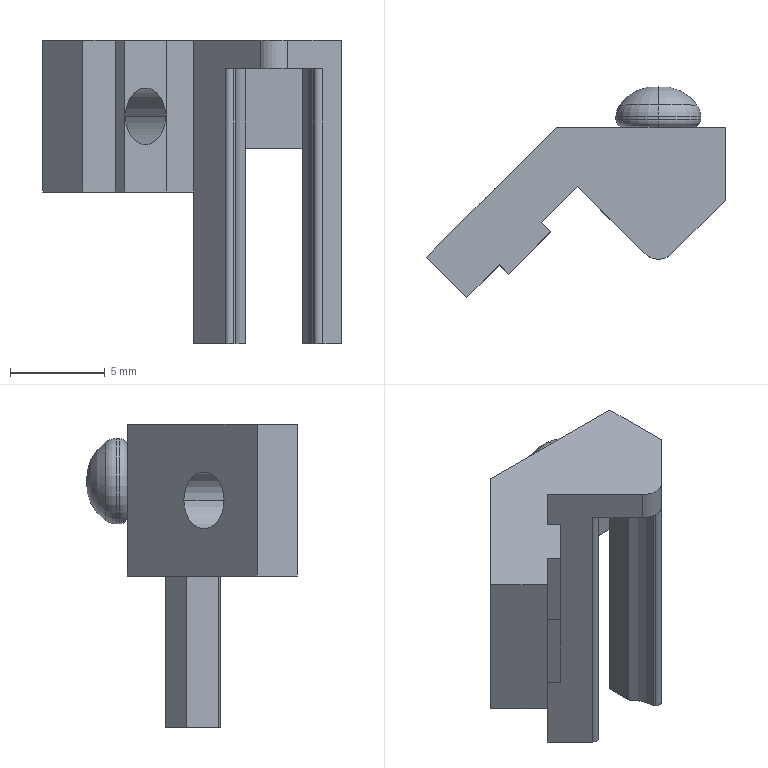Part | SolidWorks | features RefAxis 6, ICE 4, 3DProfileFeature 2, Extrusion 1, RevCut 1, Revolution 1 | 1 solid | 43 faces | box 15.769 x 11.133 x 16 mm | volume 523.118 mm3 | plane 28 | cylinder 9 | torus 6 | commonest cylinder face diameters 0.6 x2 3 x2 4.15 x2 4.5 x2 2 x1
STEP:
#1=CARTESIAN_POINT('',(0.,7.04,-1.5));
#2=VERTEX_POINT('',#1);
#3=CARTESIAN_POINT('',(0.,6.061,-3.557));
#4=VERTEX_POINT('',#3);
#5=CARTESIAN_POINT('',(0.,4.642,-1.62));
#6=DIRECTION('',(-1.,0.,0.));
#7=DIRECTION('',(0.,0.,1.));
#8=AXIS2_PLACEMENT_3D('',#5,#6,#7);
#9=CIRCLE('',#8,2.401);
#10=EDGE_CURVE('',#2,#4,#9,.T.);
#11=ORIENTED_EDGE('',*,*,#10,.F.);
#12=CARTESIAN_POINT('',(0.,6.061,0.5566));
#13=VERTEX_POINT('',#12);
#14=CARTESIAN_POINT('',(0.,4.642,-1.38));
#15=DIRECTION('',(1.,0.,0.));
#16=DIRECTION('',(0.,0.,-1.));
#17=AXIS2_PLACEMENT_3D('',#14,#15,#16);
#18=CIRCLE('',#17,2.401);
#19=EDGE_CURVE('',#2,#13,#18,.T.);
#20=ORIENTED_EDGE('',*,*,#19,.T.);
#21=CARTESIAN_POINT('',(0.,6.061,-1.5));
#22=DIRECTION('',(0.,-1.,0.));
#23=DIRECTION('',(0.,0.,-1.));
#24=AXIS2_PLACEMENT_3D('',#21,#22,#23);
#25=CIRCLE('',#24,2.057);
#26=EDGE_CURVE('',#4,#13,#25,.T.);
#27=ORIENTED_EDGE('',*,*,#26,.F.);
#28=EDGE_LOOP('',(#11,#20,#27));
#29=FACE_OUTER_BOUND('',#28,.T.);
#30=CARTESIAN_POINT('',(0.,4.642,-1.5));
#31=DIRECTION('',(0.,-1.,0.));
#32=DIRECTION('',(0.,0.,-1.));
#33=AXIS2_PLACEMENT_3D('',#30,#31,#32);
#34=TOROIDAL_SURFACE('',#33,0.1199,2.401);
#35=ADVANCED_FACE('',(#29),#34,.T.);
#36=ORIENTED_EDGE('',*,*,#26,.T.);
#37=CARTESIAN_POINT('',(0.,5.47,0.75));
#38=VERTEX_POINT('',#37);
#39=CARTESIAN_POINT('',(0.,5.47,-0.25));
#40=DIRECTION('',(1.,0.,0.));
#41=DIRECTION('',(0.,0.,-1.));
#42=AXIS2_PLACEMENT_3D('',#39,#40,#41);
#43=CIRCLE('',#42,1.);
#44=EDGE_CURVE('',#13,#38,#43,.T.);
#45=ORIENTED_EDGE('',*,*,#44,.T.);
#46=CARTESIAN_POINT('',(0.,5.47,-3.75));
#47=VERTEX_POINT('',#46);
#48=CARTESIAN_POINT('',(0.,5.47,-1.5));
#49=DIRECTION('',(0.,-1.,0.));
#50=DIRECTION('',(0.,0.,-1.));
#51=AXIS2_PLACEMENT_3D('',#48,#49,#50);
#52=CIRCLE('',#51,2.25);
#53=EDGE_CURVE('',#47,#38,#52,.T.);
#54=ORIENTED_EDGE('',*,*,#53,.F.);
#55=CARTESIAN_POINT('',(0.,5.47,-2.75));
#56=DIRECTION('',(-1.,0.,0.));
#57=DIRECTION('',(0.,0.,1.));
#58=AXIS2_PLACEMENT_3D('',#55,#56,#57);
#59=CIRCLE('',#58,1.);
#60=EDGE_CURVE('',#4,#47,#59,.T.);
#61=ORIENTED_EDGE('',*,*,#60,.F.);
#62=EDGE_LOOP('',(#36,#45,#54,#61));
#63=FACE_OUTER_BOUND('',#62,.T.);
#64=CARTESIAN_POINT('',(0.,5.47,-1.5));
#65=DIRECTION('',(0.,-1.,0.));
#66=DIRECTION('',(0.,0.,-1.));
#67=AXIS2_PLACEMENT_3D('',#64,#65,#66);
#68=TOROIDAL_SURFACE('',#67,1.25,1.);
#69=ADVANCED_FACE('',(#63),#68,.T.);
#70=ORIENTED_EDGE('',*,*,#53,.T.);
#71=CARTESIAN_POINT('',(0.,5.29,0.75));
#72=VERTEX_POINT('',#71);
#73=CARTESIAN_POINT('',(0.,7.04,0.75));
#74=DIRECTION('',(0.,-1.,0.));
#75=VECTOR('',#74,1000.);
#76=LINE('',#73,#75);
#77=EDGE_CURVE('',#38,#72,#76,.T.);
#78=ORIENTED_EDGE('',*,*,#77,.T.);
#79=CARTESIAN_POINT('',(0.,5.29,-3.75));
#80=VERTEX_POINT('',#79);
#81=CARTESIAN_POINT('',(0.,5.29,-1.5));
#82=DIRECTION('',(0.,-1.,0.));
#83=DIRECTION('',(0.,0.,-1.));
#84=AXIS2_PLACEMENT_3D('',#81,#82,#83);
#85=CIRCLE('',#84,2.25);
#86=EDGE_CURVE('',#80,#72,#85,.T.);
#87=ORIENTED_EDGE('',*,*,#86,.F.);
#88=CARTESIAN_POINT('',(0.,7.04,-3.75));
#89=DIRECTION('',(0.,-1.,0.));
#90=VECTOR('',#89,1000.);
#91=LINE('',#88,#90);
#92=EDGE_CURVE('',#47,#80,#91,.T.);
#93=ORIENTED_EDGE('',*,*,#92,.F.);
#94=EDGE_LOOP('',(#70,#78,#87,#93));
#95=FACE_OUTER_BOUND('',#94,.T.);
#96=CARTESIAN_POINT('',(0.,7.04,-1.5));
#97=DIRECTION('',(0.,-1.,0.));
#98=DIRECTION('',(0.,0.,-1.));
#99=AXIS2_PLACEMENT_3D('',#96,#97,#98);
#100=CYLINDRICAL_SURFACE('',#99,2.25);
#101=ADVANCED_FACE('',(#95),#100,.T.);
#102=ORIENTED_EDGE('',*,*,#86,.T.);
#103=CARTESIAN_POINT('',(0.,4.89,0.35));
#104=VERTEX_POINT('',#103);
#105=CARTESIAN_POINT('',(0.,5.29,0.35));
#106=DIRECTION('',(1.,0.,0.));
#107=DIRECTION('',(0.,0.,-1.));
#108=AXIS2_PLACEMENT_3D('',#105,#106,#107);
#109=CIRCLE('',#108,0.4);
#110=EDGE_CURVE('',#72,#104,#109,.T.);
#111=ORIENTED_EDGE('',*,*,#110,.T.);
#112=CARTESIAN_POINT('',(0.,4.89,-3.35));
#113=VERTEX_POINT('',#112);
#114=CARTESIAN_POINT('',(0.,4.89,-1.5));
#115=DIRECTION('',(0.,1.,0.));
#116=DIRECTION('',(0.,0.,-1.));
#117=AXIS2_PLACEMENT_3D('',#114,#115,#116);
#118=CIRCLE('',#117,1.85);
#119=EDGE_CURVE('',#104,#113,#118,.T.);
#120=ORIENTED_EDGE('',*,*,#119,.T.);
#121=CARTESIAN_POINT('',(0.,5.29,-3.35));
#122=DIRECTION('',(-1.,0.,0.));
#123=DIRECTION('',(0.,0.,1.));
#124=AXIS2_PLACEMENT_3D('',#121,#122,#123);
#125=CIRCLE('',#124,0.4);
#126=EDGE_CURVE('',#80,#113,#125,.T.);
#127=ORIENTED_EDGE('',*,*,#126,.F.);
#128=EDGE_LOOP('',(#102,#111,#120,#127));
#129=FACE_OUTER_BOUND('',#128,.T.);
#130=CARTESIAN_POINT('',(0.,5.29,-1.5));
#131=DIRECTION('',(0.,-1.,0.));
#132=DIRECTION('',(0.,0.,-1.));
#133=AXIS2_PLACEMENT_3D('',#130,#131,#132);
#134=TOROIDAL_SURFACE('',#133,1.85,0.4);
#135=ADVANCED_FACE('',(#129),#134,.T.);
#136=CARTESIAN_POINT('',(-8.355,1.905,-2.5));
#137=VERTEX_POINT('',#136);
#138=CARTESIAN_POINT('',(-10.476,-0.2162,-2.5));
#139=VERTEX_POINT('',#138);
#140=CARTESIAN_POINT('',(-9.416,0.8445,-2.5));
#141=DIRECTION('',(-0.7071,0.7071,0.));
#142=DIRECTION('',(0.7071,0.7071,0.));
#143=AXIS2_PLACEMENT_3D('',#140,#141,#142);
#144=CIRCLE('',#143,1.5);
#145=EDGE_CURVE('',#137,#139,#144,.T.);
#146=ORIENTED_EDGE('',*,*,#145,.T.);
#147=CARTESIAN_POINT('',(-7.86,-2.832,-2.5));
#148=VERTEX_POINT('',#147);
#149=CARTESIAN_POINT('',(-10.491,-0.2012,-2.5));
#150=DIRECTION('',(0.7071,-0.7071,0.));
#151=VECTOR('',#150,1000.);
#152=LINE('',#149,#151);
#153=EDGE_CURVE('',#139,#148,#152,.T.);
#154=ORIENTED_EDGE('',*,*,#153,.T.);
#155=CARTESIAN_POINT('',(-5.739,-0.7111,-2.5));
#156=VERTEX_POINT('',#155);
#157=CARTESIAN_POINT('',(-6.799,-1.772,-2.5));
#158=DIRECTION('',(0.7071,-0.7071,0.));
#159=DIRECTION('',(-0.7071,-0.7071,0.));
#160=AXIS2_PLACEMENT_3D('',#157,#158,#159);
#161=CIRCLE('',#160,1.5);
#162=EDGE_CURVE('',#148,#156,#161,.T.);
#163=ORIENTED_EDGE('',*,*,#162,.T.);
#164=CARTESIAN_POINT('',(-8.37,1.92,-2.5));
#165=DIRECTION('',(0.7071,-0.7071,0.));
#166=VECTOR('',#165,1000.);
#167=LINE('',#164,#166);
#168=EDGE_CURVE('',#137,#156,#167,.T.);
#169=ORIENTED_EDGE('',*,*,#168,.F.);
#170=EDGE_LOOP('',(#146,#154,#163,#169));
#171=FACE_OUTER_BOUND('',#170,.T.);
#172=CARTESIAN_POINT('',(-9.431,0.8595,-2.5));
#173=DIRECTION('',(0.7071,-0.7071,0.));
#174=DIRECTION('',(0.7071,0.7071,0.));
#175=AXIS2_PLACEMENT_3D('',#172,#173,#174);
#176=CYLINDRICAL_SURFACE('',#175,1.5);
#177=ADVANCED_FACE('',(#171),#176,.F.);
#178=CARTESIAN_POINT('',(0.,4.89,-1.5));
#179=DIRECTION('',(0.,1.,0.));
#180=DIRECTION('',(0.,0.,-1.));
#181=AXIS2_PLACEMENT_3D('',#178,#179,#180);
#182=CIRCLE('',#181,1.85);
#183=EDGE_CURVE('',#113,#104,#182,.T.);
#184=ORIENTED_EDGE('',*,*,#183,.F.);
#185=ORIENTED_EDGE('',*,*,#119,.F.);
#186=EDGE_LOOP('',(#184,#185));
#187=FACE_BOUND('',#186,.T.);
#188=CARTESIAN_POINT('',(3.54,4.89,1.5));
#189=VERTEX_POINT('',#188);
#190=CARTESIAN_POINT('',(3.54,4.89,-4.2));
#191=VERTEX_POINT('',#190);
#192=CARTESIAN_POINT('',(3.54,4.89,1.5));
#193=DIRECTION('',(0.,0.,-1.));
#194=VECTOR('',#193,1000.);
#195=LINE('',#192,#194);
#196=EDGE_CURVE('',#189,#191,#195,.T.);
#197=ORIENTED_EDGE('',*,*,#196,.T.);
#198=CARTESIAN_POINT('',(-5.37,4.89,-4.2));
#199=VERTEX_POINT('',#198);
#200=CARTESIAN_POINT('',(3.54,4.89,-4.2));
#201=DIRECTION('',(-1.,0.,0.));
#202=VECTOR('',#201,1000.);
#203=LINE('',#200,#202);
#204=EDGE_CURVE('',#191,#199,#203,.T.);
#205=ORIENTED_EDGE('',*,*,#204,.T.);
#206=CARTESIAN_POINT('',(-5.37,4.89,1.5));
#207=VERTEX_POINT('',#206);
#208=CARTESIAN_POINT('',(-5.37,4.89,1.5));
#209=DIRECTION('',(0.,0.,-1.));
#210=VECTOR('',#209,1000.);
#211=LINE('',#208,#210);
#212=EDGE_CURVE('',#207,#199,#211,.T.);
#213=ORIENTED_EDGE('',*,*,#212,.F.);
#214=CARTESIAN_POINT('',(3.54,4.89,1.5));
#215=DIRECTION('',(-1.,0.,0.));
#216=VECTOR('',#215,1000.);
#217=LINE('',#214,#216);
#218=EDGE_CURVE('',#189,#207,#217,.T.);
#219=ORIENTED_EDGE('',*,*,#218,.F.);
#220=EDGE_LOOP('',(#197,#205,#213,#219));
#221=FACE_OUTER_BOUND('',#220,.T.);
#222=CARTESIAN_POINT('',(3.54,4.89,1.5));
#223=DIRECTION('',(0.,-1.,0.));
#224=DIRECTION('',(0.,0.,-1.));
#225=AXIS2_PLACEMENT_3D('',#222,#223,#224);
#226=PLANE('',#225);
#227=ADVANCED_FACE('',(#187,#221),#226,.F.);
#228=CARTESIAN_POINT('',(-5.37,4.89,-6.5));
#229=VERTEX_POINT('',#228);
#230=CARTESIAN_POINT('',(-12.229,-1.969,-6.5));
#231=VERTEX_POINT('',#230);
#232=CARTESIAN_POINT('',(-5.37,4.89,-6.5));
#233=DIRECTION('',(-0.7071,-0.7071,0.));
#234=VECTOR('',#233,1000.);
#235=LINE('',#232,#234);
#236=EDGE_CURVE('',#229,#231,#235,.T.);
#237=ORIENTED_EDGE('',*,*,#236,.T.);
#238=CARTESIAN_POINT('',(-12.229,-1.969,1.5));
#239=VERTEX_POINT('',#238);
#240=CARTESIAN_POINT('',(-12.229,-1.969,1.5));
#241=DIRECTION('',(0.,0.,-1.));
#242=VECTOR('',#241,1000.);
#243=LINE('',#240,#242);
#244=EDGE_CURVE('',#239,#231,#243,.T.);
#245=ORIENTED_EDGE('',*,*,#244,.F.);
#246=CARTESIAN_POINT('',(-5.37,4.89,1.5));
#247=DIRECTION('',(-0.7071,-0.7071,0.));
#248=VECTOR('',#247,1000.);
#249=LINE('',#246,#248);
#250=EDGE_CURVE('',#207,#239,#249,.T.);
#251=ORIENTED_EDGE('',*,*,#250,.F.);
#252=ORIENTED_EDGE('',*,*,#212,.T.);
#253=CARTESIAN_POINT('',(-5.37,4.89,1.5));
#254=DIRECTION('',(0.,0.,-1.));
#255=VECTOR('',#254,1000.);
#256=LINE('',#253,#255);
#257=EDGE_CURVE('',#199,#229,#256,.T.);
#258=ORIENTED_EDGE('',*,*,#257,.T.);
#259=EDGE_LOOP('',(#237,#245,#251,#252,#258));
#260=FACE_OUTER_BOUND('',#259,.T.);
#261=ORIENTED_EDGE('',*,*,#145,.F.);
#262=CARTESIAN_POINT('',(-9.416,0.8445,-2.5));
#263=DIRECTION('',(-0.7071,0.7071,0.));
#264=DIRECTION('',(0.7071,0.7071,0.));
#265=AXIS2_PLACEMENT_3D('',#262,#263,#264);
#266=CIRCLE('',#265,1.5);
#267=EDGE_CURVE('',#139,#137,#266,.T.);
#268=ORIENTED_EDGE('',*,*,#267,.F.);
#269=EDGE_LOOP('',(#261,#268));
#270=FACE_BOUND('',#269,.T.);
#271=CARTESIAN_POINT('',(-5.37,4.89,1.5));
#272=DIRECTION('',(0.7071,-0.7071,0.));
#273=DIRECTION('',(0.7071,0.7071,0.));
#274=AXIS2_PLACEMENT_3D('',#271,#272,#273);
#275=PLANE('',#274);
#276=ADVANCED_FACE('',(#260,#270),#275,.F.);
#277=CARTESIAN_POINT('',(-7.898,-2.87,-6.5));
#278=VERTEX_POINT('',#277);
#279=CARTESIAN_POINT('',(-5.671,-0.6431,-6.5));
#280=VERTEX_POINT('',#279);
#281=CARTESIAN_POINT('',(-7.898,-2.87,-6.5));
#282=DIRECTION('',(0.7071,0.7071,0.));
#283=VECTOR('',#282,1000.);
#284=LINE('',#281,#283);
#285=EDGE_CURVE('',#278,#280,#284,.T.);
#286=ORIENTED_EDGE('',*,*,#285,.T.);
#287=CARTESIAN_POINT('',(-5.671,-0.6431,1.5));
#288=VERTEX_POINT('',#287);
#289=CARTESIAN_POINT('',(-5.671,-0.6431,1.5));
#290=DIRECTION('',(0.,0.,-1.));
#291=VECTOR('',#290,1000.);
#292=LINE('',#289,#291);
#293=EDGE_CURVE('',#288,#280,#292,.T.);
#294=ORIENTED_EDGE('',*,*,#293,.F.);
#295=CARTESIAN_POINT('',(-7.898,-2.87,1.5));
#296=VERTEX_POINT('',#295);
#297=CARTESIAN_POINT('',(-7.898,-2.87,1.5));
#298=DIRECTION('',(0.7071,0.7071,0.));
#299=VECTOR('',#298,1000.);
#300=LINE('',#297,#299);
#301=EDGE_CURVE('',#296,#288,#300,.T.);
#302=ORIENTED_EDGE('',*,*,#301,.F.);
#303=CARTESIAN_POINT('',(-7.898,-2.87,1.5));
#304=DIRECTION('',(0.,0.,-1.));
#305=VECTOR('',#304,1000.);
#306=LINE('',#303,#305);
#307=EDGE_CURVE('',#296,#278,#306,.T.);
#308=ORIENTED_EDGE('',*,*,#307,.T.);
#309=EDGE_LOOP('',(#286,#294,#302,#308));
#310=FACE_OUTER_BOUND('',#309,.T.);
#311=CARTESIAN_POINT('',(-6.799,-1.772,-2.5));
#312=DIRECTION('',(0.7071,-0.7071,0.));
#313=DIRECTION('',(-0.7071,-0.7071,0.));
#314=AXIS2_PLACEMENT_3D('',#311,#312,#313);
#315=CIRCLE('',#314,1.5);
#316=EDGE_CURVE('',#156,#148,#315,.T.);
#317=ORIENTED_EDGE('',*,*,#316,.F.);
#318=ORIENTED_EDGE('',*,*,#162,.F.);
#319=EDGE_LOOP('',(#317,#318));
#320=FACE_BOUND('',#319,.T.);
#321=CARTESIAN_POINT('',(-7.898,-2.87,1.5));
#322=DIRECTION('',(-0.7071,0.7071,0.));
#323=DIRECTION('',(-0.7071,-0.7071,0.));
#324=AXIS2_PLACEMENT_3D('',#321,#322,#323);
#325=PLANE('',#324);
#326=ADVANCED_FACE('',(#310,#320),#325,.F.);
#327=CARTESIAN_POINT('',(-3.37,2.89,-4.2));
#328=VERTEX_POINT('',#327);
#329=CARTESIAN_POINT('',(-0.24,-0.24,-4.2));
#330=DIRECTION('',(0.7071,-0.7071,0.));
#331=VECTOR('',#330,1000.);
#332=LINE('',#329,#331);
#333=EDGE_CURVE('',#199,#328,#332,.T.);
#334=ORIENTED_EDGE('',*,*,#333,.F.);
#335=ORIENTED_EDGE('',*,*,#204,.F.);
#336=CARTESIAN_POINT('',(3.54,2.89,-4.2));
#337=VERTEX_POINT('',#336);
#338=CARTESIAN_POINT('',(3.54,2.89,-4.2));
#339=DIRECTION('',(0.,1.,0.));
#340=VECTOR('',#339,1000.);
#341=LINE('',#338,#340);
#342=EDGE_CURVE('',#337,#191,#341,.T.);
#343=ORIENTED_EDGE('',*,*,#342,.F.);
#344=CARTESIAN_POINT('',(1.5,2.89,-4.2));
#345=VERTEX_POINT('',#344);
#346=CARTESIAN_POINT('',(-5.37,2.89,-4.2));
#347=DIRECTION('',(1.,0.,0.));
#348=VECTOR('',#347,1000.);
#349=LINE('',#346,#348);
#350=EDGE_CURVE('',#345,#337,#349,.T.);
#351=ORIENTED_EDGE('',*,*,#350,.F.);
#352=CARTESIAN_POINT('',(-1.5,2.89,-4.2));
#353=VERTEX_POINT('',#352);
#354=CARTESIAN_POINT('',(-5.37,2.89,-4.2));
#355=DIRECTION('',(1.,0.,0.));
#356=VECTOR('',#355,1000.);
#357=LINE('',#354,#356);
#358=EDGE_CURVE('',#353,#345,#357,.T.);
#359=ORIENTED_EDGE('',*,*,#358,.F.);
#360=CARTESIAN_POINT('',(-3.127,2.89,-4.2));
#361=VERTEX_POINT('',#360);
#362=CARTESIAN_POINT('',(-5.37,2.89,-4.2));
#363=DIRECTION('',(1.,0.,0.));
#364=VECTOR('',#363,1000.);
#365=LINE('',#362,#364);
#366=EDGE_CURVE('',#361,#353,#365,.T.);
#367=ORIENTED_EDGE('',*,*,#366,.F.);
#368=CARTESIAN_POINT('',(-5.37,2.89,-4.2));
#369=DIRECTION('',(1.,0.,0.));
#370=VECTOR('',#369,1000.);
#371=LINE('',#368,#370);
#372=EDGE_CURVE('',#328,#361,#371,.T.);
#373=ORIENTED_EDGE('',*,*,#372,.F.);
#374=EDGE_LOOP('',(#334,#335,#343,#351,#359,#367,#373));
#375=FACE_OUTER_BOUND('',#374,.T.);
#376=CARTESIAN_POINT('',(0.,0.,-4.2));
#377=DIRECTION('',(0.,0.,1.));
#378=DIRECTION('',(1.,0.,0.));
#379=AXIS2_PLACEMENT_3D('',#376,#377,#378);
#380=PLANE('',#379);
#381=ADVANCED_FACE('',(#375),#380,.F.);
#382=CARTESIAN_POINT('',(-3.249,2.769,0.));
#383=VERTEX_POINT('',#382);
#384=CARTESIAN_POINT('',(-3.249,2.769,-6.5));
#385=VERTEX_POINT('',#384);
#386=CARTESIAN_POINT('',(-3.249,2.769,1.5));
#387=DIRECTION('',(0.,0.,-1.));
#388=VECTOR('',#387,1000.);
#389=LINE('',#386,#388);
#390=EDGE_CURVE('',#383,#385,#389,.T.);
#391=ORIENTED_EDGE('',*,*,#390,.F.);
#392=CARTESIAN_POINT('',(-3.127,2.89,0.));
#393=VERTEX_POINT('',#392);
#394=CARTESIAN_POINT('',(-5.37,0.6474,0.));
#395=DIRECTION('',(0.7071,0.7071,0.));
#396=VECTOR('',#395,1000.);
#397=LINE('',#394,#396);
#398=EDGE_CURVE('',#383,#393,#397,.T.);
#399=ORIENTED_EDGE('',*,*,#398,.T.);
#400=CARTESIAN_POINT('',(-3.127,2.89,-14.5));
#401=DIRECTION('',(0.,0.,1.));
#402=VECTOR('',#401,1000.);
#403=LINE('',#400,#402);
#404=EDGE_CURVE('',#361,#393,#403,.T.);
#405=ORIENTED_EDGE('',*,*,#404,.F.);
#406=CARTESIAN_POINT('',(-3.127,2.89,-14.5));
#407=VERTEX_POINT('',#406);
#408=CARTESIAN_POINT('',(-3.127,2.89,-14.5));
#409=DIRECTION('',(0.,0.,1.));
#410=VECTOR('',#409,1000.);
#411=LINE('',#408,#410);
#412=EDGE_CURVE('',#407,#361,#411,.T.);
#413=ORIENTED_EDGE('',*,*,#412,.F.);
#414=CARTESIAN_POINT('',(-4.259,1.759,-14.5));
#415=VERTEX_POINT('',#414);
#416=CARTESIAN_POINT('',(-5.37,0.6474,-14.5));
#417=DIRECTION('',(0.7071,0.7071,0.));
#418=VECTOR('',#417,1000.);
#419=LINE('',#416,#418);
#420=EDGE_CURVE('',#415,#407,#419,.T.);
#421=ORIENTED_EDGE('',*,*,#420,.F.);
#422=CARTESIAN_POINT('',(-4.259,1.759,-6.5));
#423=VERTEX_POINT('',#422);
#424=CARTESIAN_POINT('',(-4.259,1.759,1.5));
#425=DIRECTION('',(0.,0.,-1.));
#426=VECTOR('',#425,1000.);
#427=LINE('',#424,#426);
#428=EDGE_CURVE('',#423,#415,#427,.T.);
#429=ORIENTED_EDGE('',*,*,#428,.F.);
#430=CARTESIAN_POINT('',(-6.165,-0.1481,-6.5));
#431=DIRECTION('',(0.7071,0.7071,0.));
#432=VECTOR('',#431,1000.);
#433=LINE('',#430,#432);
#434=EDGE_CURVE('',#423,#385,#433,.T.);
#435=ORIENTED_EDGE('',*,*,#434,.T.);
#436=EDGE_LOOP('',(#391,#399,#405,#413,#421,#429,#435));
#437=FACE_OUTER_BOUND('',#436,.T.);
#438=CARTESIAN_POINT('',(-5.37,0.6474,-14.5));
#439=DIRECTION('',(0.7071,-0.7071,0.));
#440=DIRECTION('',(0.7071,0.7071,0.));
#441=AXIS2_PLACEMENT_3D('',#438,#439,#440);
#442=PLANE('',#441);
#443=ADVANCED_FACE('',(#437),#442,.F.);
#444=CARTESIAN_POINT('',(-3.37,2.89,0.));
#445=VERTEX_POINT('',#444);
#446=CARTESIAN_POINT('',(-3.37,2.89,-14.5));
#447=DIRECTION('',(0.,0.,1.));
#448=VECTOR('',#447,1000.);
#449=LINE('',#446,#448);
#450=EDGE_CURVE('',#328,#445,#449,.T.);
#451=ORIENTED_EDGE('',*,*,#450,.F.);
#452=ORIENTED_EDGE('',*,*,#372,.T.);
#453=ORIENTED_EDGE('',*,*,#404,.T.);
#454=CARTESIAN_POINT('',(-3.127,2.89,0.));
#455=DIRECTION('',(-1.,0.,0.));
#456=VECTOR('',#455,1000.);
#457=LINE('',#454,#456);
#458=EDGE_CURVE('',#393,#445,#457,.T.);
#459=ORIENTED_EDGE('',*,*,#458,.T.);
#460=EDGE_LOOP('',(#451,#452,#453,#459));
#461=FACE_OUTER_BOUND('',#460,.T.);
#462=CARTESIAN_POINT('',(-3.127,2.89,-14.5));
#463=DIRECTION('',(0.,1.,0.));
#464=DIRECTION('',(-1.,0.,0.));
#465=AXIS2_PLACEMENT_3D('',#462,#463,#464);
#466=PLANE('',#465);
#467=ADVANCED_FACE('',(#461),#466,.F.);
#468=ORIENTED_EDGE('',*,*,#398,.F.);
#469=CARTESIAN_POINT('',(-0.24,-0.24,0.));
#470=DIRECTION('',(-0.7071,0.7071,0.));
#471=VECTOR('',#470,1000.);
#472=LINE('',#469,#471);
#473=EDGE_CURVE('',#383,#445,#472,.T.);
#474=ORIENTED_EDGE('',*,*,#473,.T.);
#475=ORIENTED_EDGE('',*,*,#458,.F.);
#476=EDGE_LOOP('',(#468,#474,#475));
#477=FACE_OUTER_BOUND('',#476,.T.);
#478=CARTESIAN_POINT('',(0.,0.,0.));
#479=DIRECTION('',(0.,0.,-1.));
#480=DIRECTION('',(-1.,0.,0.));
#481=AXIS2_PLACEMENT_3D('',#478,#479,#480);
#482=PLANE('',#481);
#483=ADVANCED_FACE('',(#477),#482,.T.);
#484=CARTESIAN_POINT('',(-6.165,-0.1481,1.5));
#485=VERTEX_POINT('',#484);
#486=CARTESIAN_POINT('',(-4.259,1.759,1.5));
#487=VERTEX_POINT('',#486);
#488=CARTESIAN_POINT('',(-5.37,0.6474,1.5));
#489=DIRECTION('',(0.7071,0.7071,0.));
#490=VECTOR('',#489,1000.);
#491=LINE('',#488,#490);
#492=EDGE_CURVE('',#485,#487,#491,.T.);
#493=ORIENTED_EDGE('',*,*,#492,.F.);
#494=CARTESIAN_POINT('',(-6.165,-0.1481,-6.5));
#495=VERTEX_POINT('',#494);
#496=CARTESIAN_POINT('',(-6.165,-0.1481,1.5));
#497=DIRECTION('',(0.,0.,-1.));
#498=VECTOR('',#497,1000.);
#499=LINE('',#496,#498);
#500=EDGE_CURVE('',#485,#495,#499,.T.);
#501=ORIENTED_EDGE('',*,*,#500,.T.);
#502=CARTESIAN_POINT('',(-6.165,-0.1481,-6.5));
#503=DIRECTION('',(0.7071,0.7071,0.));
#504=VECTOR('',#503,1000.);
#505=LINE('',#502,#504);
#506=EDGE_CURVE('',#495,#423,#505,.T.);
#507=ORIENTED_EDGE('',*,*,#506,.T.);
#508=CARTESIAN_POINT('',(-4.259,1.759,1.5));
#509=DIRECTION('',(0.,0.,-1.));
#510=VECTOR('',#509,1000.);
#511=LINE('',#508,#510);
#512=EDGE_CURVE('',#487,#423,#511,.T.);
#513=ORIENTED_EDGE('',*,*,#512,.F.);
#514=EDGE_LOOP('',(#493,#501,#507,#513));
#515=FACE_OUTER_BOUND('',#514,.T.);
#516=CARTESIAN_POINT('',(-5.37,0.6474,1.5));
#517=DIRECTION('',(-0.7071,0.7071,0.));
#518=DIRECTION('',(-0.7071,-0.7071,0.));
#519=AXIS2_PLACEMENT_3D('',#516,#517,#518);
#520=PLANE('',#519);
#521=ADVANCED_FACE('',(#515),#520,.F.);
#522=CARTESIAN_POINT('',(-2.567,0.06727,-14.5));
#523=VERTEX_POINT('',#522);
#524=CARTESIAN_POINT('',(-4.259,1.759,-14.5));
#525=DIRECTION('',(0.7071,-0.7071,0.));
#526=VECTOR('',#525,1000.);
#527=LINE('',#524,#526);
#528=EDGE_CURVE('',#415,#523,#527,.T.);
#529=ORIENTED_EDGE('',*,*,#528,.F.);
#530=ORIENTED_EDGE('',*,*,#420,.T.);
#531=CARTESIAN_POINT('',(-1.5,2.89,-14.5));
#532=VERTEX_POINT('',#531);
#533=CARTESIAN_POINT('',(-5.37,2.89,-14.5));
#534=DIRECTION('',(1.,0.,0.));
#535=VECTOR('',#534,1000.);
#536=LINE('',#533,#535);
#537=EDGE_CURVE('',#407,#532,#536,.T.);
#538=ORIENTED_EDGE('',*,*,#537,.T.);
#539=CARTESIAN_POINT('',(-1.5,1.434,-14.5));
#540=VERTEX_POINT('',#539);
#541=CARTESIAN_POINT('',(-1.5,2.89,-14.5));
#542=DIRECTION('',(0.,-1.,0.));
#543=VECTOR('',#542,1000.);
#544=LINE('',#541,#543);
#545=EDGE_CURVE('',#532,#540,#544,.T.);
#546=ORIENTED_EDGE('',*,*,#545,.T.);
#547=CARTESIAN_POINT('',(-2.07,0.14,-14.5));
#548=VERTEX_POINT('',#547);
#549=CARTESIAN_POINT('',(0.,0.,-14.5));
#550=DIRECTION('',(0.,0.,1.));
#551=DIRECTION('',(1.,0.,0.));
#552=AXIS2_PLACEMENT_3D('',#549,#550,#551);
#553=CIRCLE('',#552,2.075);
#554=EDGE_CURVE('',#540,#548,#553,.T.);
#555=ORIENTED_EDGE('',*,*,#554,.T.);
#556=CARTESIAN_POINT('',(-2.143,0.06727,-14.5));
#557=VERTEX_POINT('',#556);
#558=CARTESIAN_POINT('',(-2.07,0.14,-14.5));
#559=DIRECTION('',(-0.7071,-0.7071,0.));
#560=VECTOR('',#559,1000.);
#561=LINE('',#558,#560);
#562=EDGE_CURVE('',#548,#557,#561,.T.);
#563=ORIENTED_EDGE('',*,*,#562,.T.);
#564=CARTESIAN_POINT('',(-2.355,0.2794,-14.5));
#565=DIRECTION('',(0.,0.,-1.));
#566=DIRECTION('',(-1.,0.,0.));
#567=AXIS2_PLACEMENT_3D('',#564,#565,#566);
#568=CIRCLE('',#567,0.3);
#569=EDGE_CURVE('',#557,#523,#568,.T.);
#570=ORIENTED_EDGE('',*,*,#569,.T.);
#571=EDGE_LOOP('',(#529,#530,#538,#546,#555,#563,#570));
#572=FACE_OUTER_BOUND('',#571,.T.);
#573=CARTESIAN_POINT('',(0.,-1.086,-14.5));
#574=DIRECTION('',(0.,0.,1.));
#575=DIRECTION('',(1.,0.,0.));
#576=AXIS2_PLACEMENT_3D('',#573,#574,#575);
#577=PLANE('',#576);
#578=ADVANCED_FACE('',(#572),#577,.F.);
#579=CARTESIAN_POINT('',(0.7071,-1.793,0.));
#580=VERTEX_POINT('',#579);
#581=CARTESIAN_POINT('',(-0.7071,-1.793,0.));
#582=VERTEX_POINT('',#581);
#583=CARTESIAN_POINT('',(0.,-1.086,0.));
#584=DIRECTION('',(0.,0.,-1.));
#585=DIRECTION('',(-1.,0.,0.));
#586=AXIS2_PLACEMENT_3D('',#583,#584,#585);
#587=CIRCLE('',#586,1.);
#588=EDGE_CURVE('',#580,#582,#587,.T.);
#589=ORIENTED_EDGE('',*,*,#588,.F.);
#590=CARTESIAN_POINT('',(0.7071,-1.793,1.5));
#591=VERTEX_POINT('',#590);
#592=CARTESIAN_POINT('',(0.7071,-1.793,1.5));
#593=DIRECTION('',(0.,0.,-1.));
#594=VECTOR('',#593,1000.);
#595=LINE('',#592,#594);
#596=EDGE_CURVE('',#591,#580,#595,.T.);
#597=ORIENTED_EDGE('',*,*,#596,.F.);
#598=CARTESIAN_POINT('',(-0.7071,-1.793,1.5));
#599=VERTEX_POINT('',#598);
#600=CARTESIAN_POINT('',(0.,-1.086,1.5));
#601=DIRECTION('',(0.,0.,1.));
#602=DIRECTION('',(1.,0.,0.));
#603=AXIS2_PLACEMENT_3D('',#600,#601,#602);
#604=CIRCLE('',#603,1.);
#605=EDGE_CURVE('',#599,#591,#604,.T.);
#606=ORIENTED_EDGE('',*,*,#605,.F.);
#607=CARTESIAN_POINT('',(-0.7071,-1.793,1.5));
#608=DIRECTION('',(0.,0.,-1.));
#609=VECTOR('',#608,1000.);
#610=LINE('',#607,#609);
#611=EDGE_CURVE('',#599,#582,#610,.T.);
#612=ORIENTED_EDGE('',*,*,#611,.T.);
#613=EDGE_LOOP('',(#589,#597,#606,#612));
#614=FACE_OUTER_BOUND('',#613,.T.);
#615=CARTESIAN_POINT('',(0.,-1.086,1.5));
#616=DIRECTION('',(0.,0.,-1.));
#617=DIRECTION('',(-1.,0.,0.));
#618=AXIS2_PLACEMENT_3D('',#615,#616,#617);
#619=CYLINDRICAL_SURFACE('',#618,1.);
#620=ADVANCED_FACE('',(#614),#619,.T.);
#621=ORIENTED_EDGE('',*,*,#412,.T.);
#622=ORIENTED_EDGE('',*,*,#366,.T.);
#623=CARTESIAN_POINT('',(-1.5,2.89,-14.5));
#624=DIRECTION('',(0.,0.,1.));
#625=VECTOR('',#624,1000.);
#626=LINE('',#623,#625);
#627=EDGE_CURVE('',#532,#353,#626,.T.);
#628=ORIENTED_EDGE('',*,*,#627,.F.);
#629=ORIENTED_EDGE('',*,*,#537,.F.);
#630=EDGE_LOOP('',(#621,#622,#628,#629));
#631=FACE_OUTER_BOUND('',#630,.T.);
#632=CARTESIAN_POINT('',(-5.37,2.89,-4.2));
#633=DIRECTION('',(0.,1.,0.));
#634=DIRECTION('',(0.,0.,1.));
#635=AXIS2_PLACEMENT_3D('',#632,#633,#634);
#636=PLANE('',#635);
#637=ADVANCED_FACE('',(#631),#636,.T.);
#638=CARTESIAN_POINT('',(3.54,2.89,-14.5));
#639=VERTEX_POINT('',#638);
#640=CARTESIAN_POINT('',(3.54,2.89,-4.2));
#641=DIRECTION('',(0.,0.,-1.));
#642=VECTOR('',#641,1000.);
#643=LINE('',#640,#642);
#644=EDGE_CURVE('',#337,#639,#643,.T.);
#645=ORIENTED_EDGE('',*,*,#644,.F.);
#646=ORIENTED_EDGE('',*,*,#342,.T.);
#647=ORIENTED_EDGE('',*,*,#196,.F.);
#648=CARTESIAN_POINT('',(3.54,1.04,1.5));
#649=VERTEX_POINT('',#648);
#650=CARTESIAN_POINT('',(3.54,1.04,1.5));
#651=DIRECTION('',(0.,1.,0.));
#652=VECTOR('',#651,1000.);
#653=LINE('',#650,#652);
#654=EDGE_CURVE('',#649,#189,#653,.T.);
#655=ORIENTED_EDGE('',*,*,#654,.F.);
#656=CARTESIAN_POINT('',(3.54,1.04,-14.5));
#657=VERTEX_POINT('',#656);
#658=CARTESIAN_POINT('',(3.54,1.04,1.5));
#659=DIRECTION('',(0.,0.,-1.));
#660=VECTOR('',#659,1000.);
#661=LINE('',#658,#660);
#662=EDGE_CURVE('',#649,#657,#661,.T.);
#663=ORIENTED_EDGE('',*,*,#662,.T.);
#664=CARTESIAN_POINT('',(3.54,1.04,-14.5));
#665=DIRECTION('',(0.,1.,0.));
#666=VECTOR('',#665,1000.);
#667=LINE('',#664,#666);
#668=EDGE_CURVE('',#657,#639,#667,.T.);
#669=ORIENTED_EDGE('',*,*,#668,.T.);
#670=EDGE_LOOP('',(#645,#646,#647,#655,#663,#669));
#671=FACE_OUTER_BOUND('',#670,.T.);
#672=CARTESIAN_POINT('',(3.54,1.04,1.5));
#673=DIRECTION('',(-1.,0.,0.));
#674=DIRECTION('',(0.,0.,1.));
#675=AXIS2_PLACEMENT_3D('',#672,#673,#674);
#676=PLANE('',#675);
#677=ADVANCED_FACE('',(#671),#676,.F.);
#678=CARTESIAN_POINT('',(2.07,0.14,-14.5));
#679=VERTEX_POINT('',#678);
#680=CARTESIAN_POINT('',(1.5,1.434,-14.5));
#681=VERTEX_POINT('',#680);
#682=CARTESIAN_POINT('',(0.,0.,-14.5));
#683=DIRECTION('',(0.,0.,1.));
#684=DIRECTION('',(1.,0.,0.));
#685=AXIS2_PLACEMENT_3D('',#682,#683,#684);
#686=CIRCLE('',#685,2.075);
#687=EDGE_CURVE('',#679,#681,#686,.T.);
#688=ORIENTED_EDGE('',*,*,#687,.T.);
#689=CARTESIAN_POINT('',(1.5,2.89,-14.5));
#690=VERTEX_POINT('',#689);
#691=CARTESIAN_POINT('',(1.5,1.434,-14.5));
#692=DIRECTION('',(0.,1.,0.));
#693=VECTOR('',#692,1000.);
#694=LINE('',#691,#693);
#695=EDGE_CURVE('',#681,#690,#694,.T.);
#696=ORIENTED_EDGE('',*,*,#695,.T.);
#697=CARTESIAN_POINT('',(-5.37,2.89,-14.5));
#698=DIRECTION('',(1.,0.,0.));
#699=VECTOR('',#698,1000.);
#700=LINE('',#697,#699);
#701=EDGE_CURVE('',#690,#639,#700,.T.);
#702=ORIENTED_EDGE('',*,*,#701,.T.);
#703=ORIENTED_EDGE('',*,*,#668,.F.);
#704=CARTESIAN_POINT('',(2.567,0.06727,-14.5));
#705=VERTEX_POINT('',#704);
#706=CARTESIAN_POINT('',(0.7071,-1.793,-14.5));
#707=DIRECTION('',(0.7071,0.7071,0.));
#708=VECTOR('',#707,1000.);
#709=LINE('',#706,#708);
#710=EDGE_CURVE('',#705,#657,#709,.T.);
#711=ORIENTED_EDGE('',*,*,#710,.F.);
#712=CARTESIAN_POINT('',(2.143,0.06727,-14.5));
#713=VERTEX_POINT('',#712);
#714=CARTESIAN_POINT('',(2.355,0.2794,-14.5));
#715=DIRECTION('',(0.,0.,-1.));
#716=DIRECTION('',(-1.,0.,0.));
#717=AXIS2_PLACEMENT_3D('',#714,#715,#716);
#718=CIRCLE('',#717,0.3);
#719=EDGE_CURVE('',#705,#713,#718,.T.);
#720=ORIENTED_EDGE('',*,*,#719,.T.);
#721=CARTESIAN_POINT('',(2.143,0.06727,-14.5));
#722=DIRECTION('',(-0.7071,0.7071,0.));
#723=VECTOR('',#722,1000.);
#724=LINE('',#721,#723);
#725=EDGE_CURVE('',#713,#679,#724,.T.);
#726=ORIENTED_EDGE('',*,*,#725,.T.);
#727=EDGE_LOOP('',(#688,#696,#702,#703,#711,#720,#726));
#728=FACE_OUTER_BOUND('',#727,.T.);
#729=CARTESIAN_POINT('',(0.,-1.086,-14.5));
#730=DIRECTION('',(0.,0.,1.));
#731=DIRECTION('',(1.,0.,0.));
#732=AXIS2_PLACEMENT_3D('',#729,#730,#731);
#733=PLANE('',#732);
#734=ADVANCED_FACE('',(#728),#733,.F.);
#735=ORIENTED_EDGE('',*,*,#528,.T.);
#736=CARTESIAN_POINT('',(-2.567,0.06727,0.));
#737=VERTEX_POINT('',#736);
#738=CARTESIAN_POINT('',(-2.567,0.06727,-14.5));
#739=DIRECTION('',(0.,0.,1.));
#740=VECTOR('',#739,1000.);
#741=LINE('',#738,#740);
#742=EDGE_CURVE('',#523,#737,#741,.T.);
#743=ORIENTED_EDGE('',*,*,#742,.T.);
#744=CARTESIAN_POINT('',(-4.259,1.759,0.));
#745=DIRECTION('',(-0.7071,0.7071,0.));
#746=VECTOR('',#745,1000.);
#747=LINE('',#744,#746);
#748=EDGE_CURVE('',#582,#737,#747,.T.);
#749=ORIENTED_EDGE('',*,*,#748,.F.);
#750=ORIENTED_EDGE('',*,*,#611,.F.);
#751=CARTESIAN_POINT('',(-4.259,1.759,1.5));
#752=DIRECTION('',(0.7071,-0.7071,0.));
#753=VECTOR('',#752,1000.);
#754=LINE('',#751,#753);
#755=EDGE_CURVE('',#487,#599,#754,.T.);
#756=ORIENTED_EDGE('',*,*,#755,.F.);
#757=ORIENTED_EDGE('',*,*,#512,.T.);
#758=ORIENTED_EDGE('',*,*,#428,.T.);
#759=EDGE_LOOP('',(#735,#743,#749,#750,#756,#757,#758));
#760=FACE_OUTER_BOUND('',#759,.T.);
#761=CARTESIAN_POINT('',(-4.259,1.759,1.5));
#762=DIRECTION('',(0.7071,0.7071,0.));
#763=DIRECTION('',(-0.7071,0.7071,0.));
#764=AXIS2_PLACEMENT_3D('',#761,#762,#763);
#765=PLANE('',#764);
#766=ADVANCED_FACE('',(#760),#765,.F.);
#767=ORIENTED_EDGE('',*,*,#710,.T.);
#768=ORIENTED_EDGE('',*,*,#662,.F.);
#769=CARTESIAN_POINT('',(0.7071,-1.793,1.5));
#770=DIRECTION('',(0.7071,0.7071,0.));
#771=VECTOR('',#770,1000.);
#772=LINE('',#769,#771);
#773=EDGE_CURVE('',#591,#649,#772,.T.);
#774=ORIENTED_EDGE('',*,*,#773,.F.);
#775=ORIENTED_EDGE('',*,*,#596,.T.);
#776=CARTESIAN_POINT('',(2.567,0.06727,0.));
#777=VERTEX_POINT('',#776);
#778=CARTESIAN_POINT('',(0.7071,-1.793,0.));
#779=DIRECTION('',(-0.7071,-0.7071,0.));
#780=VECTOR('',#779,1000.);
#781=LINE('',#778,#780);
#782=EDGE_CURVE('',#777,#580,#781,.T.);
#783=ORIENTED_EDGE('',*,*,#782,.F.);
#784=CARTESIAN_POINT('',(2.567,0.06727,-14.5));
#785=DIRECTION('',(0.,0.,1.));
#786=VECTOR('',#785,1000.);
#787=LINE('',#784,#786);
#788=EDGE_CURVE('',#705,#777,#787,.T.);
#789=ORIENTED_EDGE('',*,*,#788,.F.);
#790=EDGE_LOOP('',(#767,#768,#774,#775,#783,#789));
#791=FACE_OUTER_BOUND('',#790,.T.);
#792=CARTESIAN_POINT('',(0.7071,-1.793,1.5));
#793=DIRECTION('',(-0.7071,0.7071,0.));
#794=DIRECTION('',(-0.7071,-0.7071,0.));
#795=AXIS2_PLACEMENT_3D('',#792,#793,#794);
#796=PLANE('',#795);
#797=ADVANCED_FACE('',(#791),#796,.F.);
#798=ORIENTED_EDGE('',*,*,#492,.T.);
#799=ORIENTED_EDGE('',*,*,#755,.T.);
#800=ORIENTED_EDGE('',*,*,#605,.T.);
#801=ORIENTED_EDGE('',*,*,#773,.T.);
#802=ORIENTED_EDGE('',*,*,#654,.T.);
#803=ORIENTED_EDGE('',*,*,#218,.T.);
#804=ORIENTED_EDGE('',*,*,#250,.T.);
#805=CARTESIAN_POINT('',(-10.108,-4.09,1.5));
#806=VERTEX_POINT('',#805);
#807=CARTESIAN_POINT('',(-12.229,-1.969,1.5));
#808=DIRECTION('',(0.7071,-0.7071,0.));
#809=VECTOR('',#808,1000.);
#810=LINE('',#807,#809);
#811=EDGE_CURVE('',#239,#806,#810,.T.);
#812=ORIENTED_EDGE('',*,*,#811,.T.);
#813=CARTESIAN_POINT('',(-8.393,-2.376,1.5));
#814=VERTEX_POINT('',#813);
#815=CARTESIAN_POINT('',(-10.108,-4.09,1.5));
#816=DIRECTION('',(0.7071,0.7071,0.));
#817=VECTOR('',#816,1000.);
#818=LINE('',#815,#817);
#819=EDGE_CURVE('',#806,#814,#818,.T.);
#820=ORIENTED_EDGE('',*,*,#819,.T.);
#821=CARTESIAN_POINT('',(-8.393,-2.376,1.5));
#822=DIRECTION('',(0.7071,-0.7071,0.));
#823=VECTOR('',#822,1000.);
#824=LINE('',#821,#823);
#825=EDGE_CURVE('',#814,#296,#824,.T.);
#826=ORIENTED_EDGE('',*,*,#825,.T.);
#827=ORIENTED_EDGE('',*,*,#301,.T.);
#828=CARTESIAN_POINT('',(-5.671,-0.6431,1.5));
#829=DIRECTION('',(-0.7071,0.7071,0.));
#830=VECTOR('',#829,1000.);
#831=LINE('',#828,#830);
#832=EDGE_CURVE('',#288,#485,#831,.T.);
#833=ORIENTED_EDGE('',*,*,#832,.T.);
#834=EDGE_LOOP('',(#798,#799,#800,#801,#802,#803,#804,#812,#820,#826,#827,#833));
#835=FACE_OUTER_BOUND('',#834,.T.);
#836=CARTESIAN_POINT('',(0.,-1.086,1.5));
#837=DIRECTION('',(0.,0.,1.));
#838=DIRECTION('',(1.,0.,0.));
#839=AXIS2_PLACEMENT_3D('',#836,#837,#838);
#840=PLANE('',#839);
#841=ADVANCED_FACE('',(#835),#840,.T.);
#842=CARTESIAN_POINT('',(1.5,2.89,-14.5));
#843=DIRECTION('',(0.,0.,1.));
#844=VECTOR('',#843,1000.);
#845=LINE('',#842,#844);
#846=EDGE_CURVE('',#690,#345,#845,.T.);
#847=ORIENTED_EDGE('',*,*,#846,.T.);
#848=ORIENTED_EDGE('',*,*,#350,.T.);
#849=ORIENTED_EDGE('',*,*,#644,.T.);
#850=ORIENTED_EDGE('',*,*,#701,.F.);
#851=EDGE_LOOP('',(#847,#848,#849,#850));
#852=FACE_OUTER_BOUND('',#851,.T.);
#853=CARTESIAN_POINT('',(-5.37,2.89,-4.2));
#854=DIRECTION('',(0.,1.,0.));
#855=DIRECTION('',(0.,0.,1.));
#856=AXIS2_PLACEMENT_3D('',#853,#854,#855);
#857=PLANE('',#856);
#858=ADVANCED_FACE('',(#852),#857,.T.);
#859=ORIENTED_EDGE('',*,*,#748,.T.);
#860=CARTESIAN_POINT('',(-2.143,0.06727,0.));
#861=VERTEX_POINT('',#860);
#862=CARTESIAN_POINT('',(-2.355,0.2794,0.));
#863=DIRECTION('',(0.,0.,-1.));
#864=DIRECTION('',(-1.,0.,0.));
#865=AXIS2_PLACEMENT_3D('',#862,#863,#864);
#866=CIRCLE('',#865,0.3);
#867=EDGE_CURVE('',#861,#737,#866,.T.);
#868=ORIENTED_EDGE('',*,*,#867,.F.);
#869=CARTESIAN_POINT('',(-2.07,0.14,0.));
#870=VERTEX_POINT('',#869);
#871=CARTESIAN_POINT('',(-2.07,0.14,0.));
#872=DIRECTION('',(-0.7071,-0.7071,0.));
#873=VECTOR('',#872,1000.);
#874=LINE('',#871,#873);
#875=EDGE_CURVE('',#870,#861,#874,.T.);
#876=ORIENTED_EDGE('',*,*,#875,.F.);
#877=CARTESIAN_POINT('',(-1.5,1.434,0.));
#878=VERTEX_POINT('',#877);
#879=CARTESIAN_POINT('',(0.,0.,0.));
#880=DIRECTION('',(0.,0.,1.));
#881=DIRECTION('',(1.,0.,0.));
#882=AXIS2_PLACEMENT_3D('',#879,#880,#881);
#883=CIRCLE('',#882,2.075);
#884=EDGE_CURVE('',#878,#870,#883,.T.);
#885=ORIENTED_EDGE('',*,*,#884,.F.);
#886=CARTESIAN_POINT('',(-1.5,2.89,0.));
#887=VERTEX_POINT('',#886);
#888=CARTESIAN_POINT('',(-1.5,2.89,0.));
#889=DIRECTION('',(0.,-1.,0.));
#890=VECTOR('',#889,1000.);
#891=LINE('',#888,#890);
#892=EDGE_CURVE('',#887,#878,#891,.T.);
#893=ORIENTED_EDGE('',*,*,#892,.F.);
#894=CARTESIAN_POINT('',(1.5,2.89,0.));
#895=VERTEX_POINT('',#894);
#896=CARTESIAN_POINT('',(1.5,2.89,0.));
#897=DIRECTION('',(-1.,0.,0.));
#898=VECTOR('',#897,1000.);
#899=LINE('',#896,#898);
#900=EDGE_CURVE('',#895,#887,#899,.T.);
#901=ORIENTED_EDGE('',*,*,#900,.F.);
#902=CARTESIAN_POINT('',(1.5,1.434,0.));
#903=VERTEX_POINT('',#902);
#904=CARTESIAN_POINT('',(1.5,1.434,0.));
#905=DIRECTION('',(0.,1.,0.));
#906=VECTOR('',#905,1000.);
#907=LINE('',#904,#906);
#908=EDGE_CURVE('',#903,#895,#907,.T.);
#909=ORIENTED_EDGE('',*,*,#908,.F.);
#910=CARTESIAN_POINT('',(2.07,0.14,0.));
#911=VERTEX_POINT('',#910);
#912=CARTESIAN_POINT('',(0.,0.,0.));
#913=DIRECTION('',(0.,0.,1.));
#914=DIRECTION('',(1.,0.,0.));
#915=AXIS2_PLACEMENT_3D('',#912,#913,#914);
#916=CIRCLE('',#915,2.075);
#917=EDGE_CURVE('',#911,#903,#916,.T.);
#918=ORIENTED_EDGE('',*,*,#917,.F.);
#919=CARTESIAN_POINT('',(2.143,0.06727,0.));
#920=VERTEX_POINT('',#919);
#921=CARTESIAN_POINT('',(2.143,0.06727,0.));
#922=DIRECTION('',(-0.7071,0.7071,0.));
#923=VECTOR('',#922,1000.);
#924=LINE('',#921,#923);
#925=EDGE_CURVE('',#920,#911,#924,.T.);
#926=ORIENTED_EDGE('',*,*,#925,.F.);
#927=CARTESIAN_POINT('',(2.355,0.2794,0.));
#928=DIRECTION('',(0.,0.,-1.));
#929=DIRECTION('',(-1.,0.,0.));
#930=AXIS2_PLACEMENT_3D('',#927,#928,#929);
#931=CIRCLE('',#930,0.3);
#932=EDGE_CURVE('',#777,#920,#931,.T.);
#933=ORIENTED_EDGE('',*,*,#932,.F.);
#934=ORIENTED_EDGE('',*,*,#782,.T.);
#935=ORIENTED_EDGE('',*,*,#588,.T.);
#936=EDGE_LOOP('',(#859,#868,#876,#885,#893,#901,#909,#918,#926,#933,#934,#935));
#937=FACE_OUTER_BOUND('',#936,.T.);
#938=CARTESIAN_POINT('',(2.355,0.2794,0.));
#939=DIRECTION('',(0.,0.,-1.));
#940=DIRECTION('',(-1.,0.,0.));
#941=AXIS2_PLACEMENT_3D('',#938,#939,#940);
#942=PLANE('',#941);
#943=ADVANCED_FACE('',(#937),#942,.T.);
#944=CARTESIAN_POINT('',(1.5,2.89,-14.5));
#945=DIRECTION('',(0.,0.,1.));
#946=VECTOR('',#945,1000.);
#947=LINE('',#944,#946);
#948=EDGE_CURVE('',#345,#895,#947,.T.);
#949=ORIENTED_EDGE('',*,*,#948,.T.);
#950=ORIENTED_EDGE('',*,*,#900,.T.);
#951=CARTESIAN_POINT('',(-1.5,2.89,-14.5));
#952=DIRECTION('',(0.,0.,1.));
#953=VECTOR('',#952,1000.);
#954=LINE('',#951,#953);
#955=EDGE_CURVE('',#353,#887,#954,.T.);
#956=ORIENTED_EDGE('',*,*,#955,.F.);
#957=ORIENTED_EDGE('',*,*,#358,.T.);
#958=EDGE_LOOP('',(#949,#950,#956,#957));
#959=FACE_OUTER_BOUND('',#958,.T.);
#960=CARTESIAN_POINT('',(1.5,2.89,-14.5));
#961=DIRECTION('',(0.,1.,0.));
#962=DIRECTION('',(0.,0.,1.));
#963=AXIS2_PLACEMENT_3D('',#960,#961,#962);
#964=PLANE('',#963);
#965=ADVANCED_FACE('',(#959),#964,.F.);
#966=ORIENTED_EDGE('',*,*,#867,.T.);
#967=ORIENTED_EDGE('',*,*,#742,.F.);
#968=ORIENTED_EDGE('',*,*,#569,.F.);
#969=CARTESIAN_POINT('',(-2.143,0.06727,-14.5));
#970=DIRECTION('',(0.,0.,1.));
#971=VECTOR('',#970,1000.);
#972=LINE('',#969,#971);
#973=EDGE_CURVE('',#557,#861,#972,.T.);
#974=ORIENTED_EDGE('',*,*,#973,.T.);
#975=EDGE_LOOP('',(#966,#967,#968,#974));
#976=FACE_OUTER_BOUND('',#975,.T.);
#977=CARTESIAN_POINT('',(-2.355,0.2794,-14.5));
#978=DIRECTION('',(0.,0.,1.));
#979=DIRECTION('',(1.,0.,0.));
#980=AXIS2_PLACEMENT_3D('',#977,#978,#979);
#981=CYLINDRICAL_SURFACE('',#980,0.3);
#982=ADVANCED_FACE('',(#976),#981,.T.);
#983=ORIENTED_EDGE('',*,*,#875,.T.);
#984=ORIENTED_EDGE('',*,*,#973,.F.);
#985=ORIENTED_EDGE('',*,*,#562,.F.);
#986=CARTESIAN_POINT('',(-2.07,0.14,-14.5));
#987=DIRECTION('',(0.,0.,1.));
#988=VECTOR('',#987,1000.);
#989=LINE('',#986,#988);
#990=EDGE_CURVE('',#548,#870,#989,.T.);
#991=ORIENTED_EDGE('',*,*,#990,.T.);
#992=EDGE_LOOP('',(#983,#984,#985,#991));
#993=FACE_OUTER_BOUND('',#992,.T.);
#994=CARTESIAN_POINT('',(-2.07,0.14,-14.5));
#995=DIRECTION('',(-0.7071,0.7071,0.));
#996=DIRECTION('',(-0.7071,-0.7071,0.));
#997=AXIS2_PLACEMENT_3D('',#994,#995,#996);
#998=PLANE('',#997);
#999=ADVANCED_FACE('',(#993),#998,.F.);
#1000=ORIENTED_EDGE('',*,*,#884,.T.);
#1001=ORIENTED_EDGE('',*,*,#990,.F.);
#1002=ORIENTED_EDGE('',*,*,#554,.F.);
#1003=CARTESIAN_POINT('',(-1.5,1.434,-14.5));
#1004=DIRECTION('',(0.,0.,1.));
#1005=VECTOR('',#1004,1000.);
#1006=LINE('',#1003,#1005);
#1007=EDGE_CURVE('',#540,#878,#1006,.T.);
#1008=ORIENTED_EDGE('',*,*,#1007,.T.);
#1009=EDGE_LOOP('',(#1000,#1001,#1002,#1008));
#1010=FACE_OUTER_BOUND('',#1009,.T.);
#1011=CARTESIAN_POINT('',(0.,0.,-14.5));
#1012=DIRECTION('',(0.,0.,1.));
#1013=DIRECTION('',(1.,0.,0.));
#1014=AXIS2_PLACEMENT_3D('',#1011,#1012,#1013);
#1015=CYLINDRICAL_SURFACE('',#1014,2.075);
#1016=ADVANCED_FACE('',(#1010),#1015,.F.);
#1017=ORIENTED_EDGE('',*,*,#892,.T.);
#1018=ORIENTED_EDGE('',*,*,#1007,.F.);
#1019=ORIENTED_EDGE('',*,*,#545,.F.);
#1020=ORIENTED_EDGE('',*,*,#627,.T.);
#1021=ORIENTED_EDGE('',*,*,#955,.T.);
#1022=EDGE_LOOP('',(#1017,#1018,#1019,#1020,#1021));
#1023=FACE_OUTER_BOUND('',#1022,.T.);
#1024=CARTESIAN_POINT('',(-1.5,2.89,-14.5));
#1025=DIRECTION('',(-1.,0.,0.));
#1026=DIRECTION('',(0.,-1.,0.));
#1027=AXIS2_PLACEMENT_3D('',#1024,#1025,#1026);
#1028=PLANE('',#1027);
#1029=ADVANCED_FACE('',(#1023),#1028,.F.);
#1030=ORIENTED_EDGE('',*,*,#908,.T.);
#1031=ORIENTED_EDGE('',*,*,#948,.F.);
#1032=ORIENTED_EDGE('',*,*,#846,.F.);
#1033=ORIENTED_EDGE('',*,*,#695,.F.);
#1034=CARTESIAN_POINT('',(1.5,1.434,-14.5));
#1035=DIRECTION('',(0.,0.,1.));
#1036=VECTOR('',#1035,1000.);
#1037=LINE('',#1034,#1036);
#1038=EDGE_CURVE('',#681,#903,#1037,.T.);
#1039=ORIENTED_EDGE('',*,*,#1038,.T.);
#1040=EDGE_LOOP('',(#1030,#1031,#1032,#1033,#1039));
#1041=FACE_OUTER_BOUND('',#1040,.T.);
#1042=CARTESIAN_POINT('',(1.5,1.434,-14.5));
#1043=DIRECTION('',(1.,0.,0.));
#1044=DIRECTION('',(0.,0.,-1.));
#1045=AXIS2_PLACEMENT_3D('',#1042,#1043,#1044);
#1046=PLANE('',#1045);
#1047=ADVANCED_FACE('',(#1041),#1046,.F.);
#1048=ORIENTED_EDGE('',*,*,#917,.T.);
#1049=ORIENTED_EDGE('',*,*,#1038,.F.);
#1050=ORIENTED_EDGE('',*,*,#687,.F.);
#1051=CARTESIAN_POINT('',(2.07,0.14,-14.5));
#1052=DIRECTION('',(0.,0.,1.));
#1053=VECTOR('',#1052,1000.);
#1054=LINE('',#1051,#1053);
#1055=EDGE_CURVE('',#679,#911,#1054,.T.);
#1056=ORIENTED_EDGE('',*,*,#1055,.T.);
#1057=EDGE_LOOP('',(#1048,#1049,#1050,#1056));
#1058=FACE_OUTER_BOUND('',#1057,.T.);
#1059=CARTESIAN_POINT('',(0.,0.,-14.5));
#1060=DIRECTION('',(0.,0.,1.));
#1061=DIRECTION('',(1.,0.,0.));
#1062=AXIS2_PLACEMENT_3D('',#1059,#1060,#1061);
#1063=CYLINDRICAL_SURFACE('',#1062,2.075);
#1064=ADVANCED_FACE('',(#1058),#1063,.F.);
#1065=ORIENTED_EDGE('',*,*,#925,.T.);
#1066=ORIENTED_EDGE('',*,*,#1055,.F.);
#1067=ORIENTED_EDGE('',*,*,#725,.F.);
#1068=CARTESIAN_POINT('',(2.143,0.06727,-14.5));
#1069=DIRECTION('',(0.,0.,1.));
#1070=VECTOR('',#1069,1000.);
#1071=LINE('',#1068,#1070);
#1072=EDGE_CURVE('',#713,#920,#1071,.T.);
#1073=ORIENTED_EDGE('',*,*,#1072,.T.);
#1074=EDGE_LOOP('',(#1065,#1066,#1067,#1073));
#1075=FACE_OUTER_BOUND('',#1074,.T.);
#1076=CARTESIAN_POINT('',(2.143,0.06727,-14.5));
#1077=DIRECTION('',(0.7071,0.7071,0.));
#1078=DIRECTION('',(-0.7071,0.7071,0.));
#1079=AXIS2_PLACEMENT_3D('',#1076,#1077,#1078);
#1080=PLANE('',#1079);
#1081=ADVANCED_FACE('',(#1075),#1080,.F.);
#1082=ORIENTED_EDGE('',*,*,#932,.T.);
#1083=ORIENTED_EDGE('',*,*,#1072,.F.);
#1084=ORIENTED_EDGE('',*,*,#719,.F.);
#1085=ORIENTED_EDGE('',*,*,#788,.T.);
#1086=EDGE_LOOP('',(#1082,#1083,#1084,#1085));
#1087=FACE_OUTER_BOUND('',#1086,.T.);
#1088=CARTESIAN_POINT('',(2.355,0.2794,-14.5));
#1089=DIRECTION('',(0.,0.,1.));
#1090=DIRECTION('',(1.,0.,0.));
#1091=AXIS2_PLACEMENT_3D('',#1088,#1089,#1090);
#1092=CYLINDRICAL_SURFACE('',#1091,0.3);
#1093=ADVANCED_FACE('',(#1087),#1092,.T.);
#1094=ORIENTED_EDGE('',*,*,#257,.F.);
#1095=ORIENTED_EDGE('',*,*,#333,.T.);
#1096=ORIENTED_EDGE('',*,*,#450,.T.);
#1097=ORIENTED_EDGE('',*,*,#473,.F.);
#1098=ORIENTED_EDGE('',*,*,#390,.T.);
#1099=CARTESIAN_POINT('',(-3.249,2.769,-6.5));
#1100=DIRECTION('',(-0.7071,0.7071,0.));
#1101=VECTOR('',#1100,1000.);
#1102=LINE('',#1099,#1101);
#1103=EDGE_CURVE('',#385,#229,#1102,.T.);
#1104=ORIENTED_EDGE('',*,*,#1103,.T.);
#1105=EDGE_LOOP('',(#1094,#1095,#1096,#1097,#1098,#1104));
#1106=FACE_OUTER_BOUND('',#1105,.T.);
#1107=CARTESIAN_POINT('',(-3.249,2.769,1.5));
#1108=DIRECTION('',(-0.7071,-0.7071,0.));
#1109=DIRECTION('',(0.7071,-0.7071,0.));
#1110=AXIS2_PLACEMENT_3D('',#1107,#1108,#1109);
#1111=PLANE('',#1110);
#1112=ADVANCED_FACE('',(#1106),#1111,.F.);
#1113=CARTESIAN_POINT('',(-10.108,-4.09,-6.5));
#1114=VERTEX_POINT('',#1113);
#1115=CARTESIAN_POINT('',(-12.229,-1.969,-6.5));
#1116=DIRECTION('',(0.7071,-0.7071,0.));
#1117=VECTOR('',#1116,1000.);
#1118=LINE('',#1115,#1117);
#1119=EDGE_CURVE('',#231,#1114,#1118,.T.);
#1120=ORIENTED_EDGE('',*,*,#1119,.T.);
#1121=CARTESIAN_POINT('',(-10.108,-4.09,1.5));
#1122=DIRECTION('',(0.,0.,-1.));
#1123=VECTOR('',#1122,1000.);
#1124=LINE('',#1121,#1123);
#1125=EDGE_CURVE('',#806,#1114,#1124,.T.);
#1126=ORIENTED_EDGE('',*,*,#1125,.F.);
#1127=ORIENTED_EDGE('',*,*,#811,.F.);
#1128=ORIENTED_EDGE('',*,*,#244,.T.);
#1129=EDGE_LOOP('',(#1120,#1126,#1127,#1128));
#1130=FACE_OUTER_BOUND('',#1129,.T.);
#1131=CARTESIAN_POINT('',(-12.229,-1.969,1.5));
#1132=DIRECTION('',(0.7071,0.7071,0.));
#1133=DIRECTION('',(-0.7071,0.7071,0.));
#1134=AXIS2_PLACEMENT_3D('',#1131,#1132,#1133);
#1135=PLANE('',#1134);
#1136=ADVANCED_FACE('',(#1130),#1135,.F.);
#1137=CARTESIAN_POINT('',(-8.393,-2.376,-6.5));
#1138=VERTEX_POINT('',#1137);
#1139=CARTESIAN_POINT('',(-10.108,-4.09,-6.5));
#1140=DIRECTION('',(0.7071,0.7071,0.));
#1141=VECTOR('',#1140,1000.);
#1142=LINE('',#1139,#1141);
#1143=EDGE_CURVE('',#1114,#1138,#1142,.T.);
#1144=ORIENTED_EDGE('',*,*,#1143,.T.);
#1145=CARTESIAN_POINT('',(-8.393,-2.376,1.5));
#1146=DIRECTION('',(0.,0.,-1.));
#1147=VECTOR('',#1146,1000.);
#1148=LINE('',#1145,#1147);
#1149=EDGE_CURVE('',#814,#1138,#1148,.T.);
#1150=ORIENTED_EDGE('',*,*,#1149,.F.);
#1151=ORIENTED_EDGE('',*,*,#819,.F.);
#1152=ORIENTED_EDGE('',*,*,#1125,.T.);
#1153=EDGE_LOOP('',(#1144,#1150,#1151,#1152));
#1154=FACE_OUTER_BOUND('',#1153,.T.);
#1155=CARTESIAN_POINT('',(-10.108,-4.09,1.5));
#1156=DIRECTION('',(-0.7071,0.7071,0.));
#1157=DIRECTION('',(-0.7071,-0.7071,0.));
#1158=AXIS2_PLACEMENT_3D('',#1155,#1156,#1157);
#1159=PLANE('',#1158);
#1160=ADVANCED_FACE('',(#1154),#1159,.F.);
#1161=CARTESIAN_POINT('',(-8.393,-2.376,-6.5));
#1162=DIRECTION('',(0.7071,-0.7071,0.));
#1163=VECTOR('',#1162,1000.);
#1164=LINE('',#1161,#1163);
#1165=EDGE_CURVE('',#1138,#278,#1164,.T.);
#1166=ORIENTED_EDGE('',*,*,#1165,.T.);
#1167=ORIENTED_EDGE('',*,*,#307,.F.);
#1168=ORIENTED_EDGE('',*,*,#825,.F.);
#1169=ORIENTED_EDGE('',*,*,#1149,.T.);
#1170=EDGE_LOOP('',(#1166,#1167,#1168,#1169));
#1171=FACE_OUTER_BOUND('',#1170,.T.);
#1172=CARTESIAN_POINT('',(-8.393,-2.376,1.5));
#1173=DIRECTION('',(0.7071,0.7071,0.));
#1174=DIRECTION('',(-0.7071,0.7071,0.));
#1175=AXIS2_PLACEMENT_3D('',#1172,#1173,#1174);
#1176=PLANE('',#1175);
#1177=ADVANCED_FACE('',(#1171),#1176,.F.);
#1178=CARTESIAN_POINT('',(-5.671,-0.6431,-6.5));
#1179=DIRECTION('',(-0.7071,0.7071,0.));
#1180=VECTOR('',#1179,1000.);
#1181=LINE('',#1178,#1180);
#1182=EDGE_CURVE('',#280,#495,#1181,.T.);
#1183=ORIENTED_EDGE('',*,*,#1182,.T.);
#1184=ORIENTED_EDGE('',*,*,#500,.F.);
#1185=ORIENTED_EDGE('',*,*,#832,.F.);
#1186=ORIENTED_EDGE('',*,*,#293,.T.);
#1187=EDGE_LOOP('',(#1183,#1184,#1185,#1186));
#1188=FACE_OUTER_BOUND('',#1187,.T.);
#1189=CARTESIAN_POINT('',(-5.671,-0.6431,1.5));
#1190=DIRECTION('',(-0.7071,-0.7071,0.));
#1191=DIRECTION('',(0.7071,-0.7071,0.));
#1192=AXIS2_PLACEMENT_3D('',#1189,#1190,#1191);
#1193=PLANE('',#1192);
#1194=ADVANCED_FACE('',(#1188),#1193,.F.);
#1195=ORIENTED_EDGE('',*,*,#236,.F.);
#1196=ORIENTED_EDGE('',*,*,#1103,.F.);
#1197=ORIENTED_EDGE('',*,*,#434,.F.);
#1198=ORIENTED_EDGE('',*,*,#506,.F.);
#1199=ORIENTED_EDGE('',*,*,#1182,.F.);
#1200=ORIENTED_EDGE('',*,*,#285,.F.);
#1201=ORIENTED_EDGE('',*,*,#1165,.F.);
#1202=ORIENTED_EDGE('',*,*,#1143,.F.);
#1203=ORIENTED_EDGE('',*,*,#1119,.F.);
#1204=EDGE_LOOP('',(#1195,#1196,#1197,#1198,#1199,#1200,#1201,#1202,#1203));
#1205=FACE_OUTER_BOUND('',#1204,.T.);
#1206=CARTESIAN_POINT('',(0.,0.,-6.5));
#1207=DIRECTION('',(0.,0.,1.));
#1208=DIRECTION('',(1.,0.,0.));
#1209=AXIS2_PLACEMENT_3D('',#1206,#1207,#1208);
#1210=PLANE('',#1209);
#1211=ADVANCED_FACE('',(#1205),#1210,.F.);
#1212=ORIENTED_EDGE('',*,*,#153,.F.);
#1213=ORIENTED_EDGE('',*,*,#267,.T.);
#1214=ORIENTED_EDGE('',*,*,#168,.T.);
#1215=ORIENTED_EDGE('',*,*,#316,.T.);
#1216=EDGE_LOOP('',(#1212,#1213,#1214,#1215));
#1217=FACE_OUTER_BOUND('',#1216,.T.);
#1218=CARTESIAN_POINT('',(-9.431,0.8595,-2.5));
#1219=DIRECTION('',(0.7071,-0.7071,0.));
#1220=DIRECTION('',(0.7071,0.7071,0.));
#1221=AXIS2_PLACEMENT_3D('',#1218,#1219,#1220);
#1222=CYLINDRICAL_SURFACE('',#1221,1.5);
#1223=ADVANCED_FACE('',(#1217),#1222,.F.);
#1224=ORIENTED_EDGE('',*,*,#110,.F.);
#1225=CARTESIAN_POINT('',(0.,5.29,-1.5));
#1226=DIRECTION('',(0.,-1.,0.));
#1227=DIRECTION('',(0.,0.,-1.));
#1228=AXIS2_PLACEMENT_3D('',#1225,#1226,#1227);
#1229=CIRCLE('',#1228,2.25);
#1230=EDGE_CURVE('',#72,#80,#1229,.T.);
#1231=ORIENTED_EDGE('',*,*,#1230,.T.);
#1232=ORIENTED_EDGE('',*,*,#126,.T.);
#1233=ORIENTED_EDGE('',*,*,#183,.T.);
#1234=EDGE_LOOP('',(#1224,#1231,#1232,#1233));
#1235=FACE_OUTER_BOUND('',#1234,.T.);
#1236=CARTESIAN_POINT('',(0.,5.29,-1.5));
#1237=DIRECTION('',(0.,-1.,0.));
#1238=DIRECTION('',(0.,0.,-1.));
#1239=AXIS2_PLACEMENT_3D('',#1236,#1237,#1238);
#1240=TOROIDAL_SURFACE('',#1239,1.85,0.4);
#1241=ADVANCED_FACE('',(#1235),#1240,.T.);
#1242=ORIENTED_EDGE('',*,*,#77,.F.);
#1243=CARTESIAN_POINT('',(0.,5.47,-1.5));
#1244=DIRECTION('',(0.,-1.,0.));
#1245=DIRECTION('',(0.,0.,-1.));
#1246=AXIS2_PLACEMENT_3D('',#1243,#1244,#1245);
#1247=CIRCLE('',#1246,2.25);
#1248=EDGE_CURVE('',#38,#47,#1247,.T.);
#1249=ORIENTED_EDGE('',*,*,#1248,.T.);
#1250=ORIENTED_EDGE('',*,*,#92,.T.);
#1251=ORIENTED_EDGE('',*,*,#1230,.F.);
#1252=EDGE_LOOP('',(#1242,#1249,#1250,#1251));
#1253=FACE_OUTER_BOUND('',#1252,.T.);
#1254=CARTESIAN_POINT('',(0.,7.04,-1.5));
#1255=DIRECTION('',(0.,-1.,0.));
#1256=DIRECTION('',(0.,0.,-1.));
#1257=AXIS2_PLACEMENT_3D('',#1254,#1255,#1256);
#1258=CYLINDRICAL_SURFACE('',#1257,2.25);
#1259=ADVANCED_FACE('',(#1253),#1258,.T.);
#1260=ORIENTED_EDGE('',*,*,#44,.F.);
#1261=CARTESIAN_POINT('',(0.,6.061,-1.5));
#1262=DIRECTION('',(0.,-1.,0.));
#1263=DIRECTION('',(0.,0.,-1.));
#1264=AXIS2_PLACEMENT_3D('',#1261,#1262,#1263);
#1265=CIRCLE('',#1264,2.057);
#1266=EDGE_CURVE('',#13,#4,#1265,.T.);
#1267=ORIENTED_EDGE('',*,*,#1266,.T.);
#1268=ORIENTED_EDGE('',*,*,#60,.T.);
#1269=ORIENTED_EDGE('',*,*,#1248,.F.);
#1270=EDGE_LOOP('',(#1260,#1267,#1268,#1269));
#1271=FACE_OUTER_BOUND('',#1270,.T.);
#1272=CARTESIAN_POINT('',(0.,5.47,-1.5));
#1273=DIRECTION('',(0.,-1.,0.));
#1274=DIRECTION('',(0.,0.,-1.));
#1275=AXIS2_PLACEMENT_3D('',#1272,#1273,#1274);
#1276=TOROIDAL_SURFACE('',#1275,1.25,1.);
#1277=ADVANCED_FACE('',(#1271),#1276,.T.);
#1278=ORIENTED_EDGE('',*,*,#19,.F.);
#1279=ORIENTED_EDGE('',*,*,#10,.T.);
#1280=ORIENTED_EDGE('',*,*,#1266,.F.);
#1281=EDGE_LOOP('',(#1278,#1279,#1280));
#1282=FACE_OUTER_BOUND('',#1281,.T.);
#1283=CARTESIAN_POINT('',(0.,4.642,-1.5));
#1284=DIRECTION('',(0.,-1.,0.));
#1285=DIRECTION('',(0.,0.,-1.));
#1286=AXIS2_PLACEMENT_3D('',#1283,#1284,#1285);
#1287=TOROIDAL_SURFACE('',#1286,0.1199,2.401);
#1288=ADVANCED_FACE('',(#1282),#1287,.T.);
#1289=CLOSED_SHELL('',(#35,#69,#101,#135,#177,#227,#276,#326,#381,#443,#467,#483,#521,#578,#620,#637,#677,#734,#766,#797,#841,#858,#943,#965,#982,#999,#1016,#1029,#1047,#1064,#1081,#1093,#1112,#1136,#1160,#1177,#1194,#1211,#1223,#1241,#1259,#1277,#1288));
#1290=MANIFOLD_SOLID_BREP('',#1289);
#1291=CARTESIAN_POINT('',(0.,0.,0.));
#1292=DIRECTION('',(0.,0.,1.));
#1293=DIRECTION('',(1.,0.,0.));
#1294=AXIS2_PLACEMENT_3D('',#1291,#1292,#1293);
#1295=(LENGTH_UNIT()NAMED_UNIT(*)SI_UNIT(.MILLI.,.METRE.));
#1296=UNCERTAINTY_MEASURE_WITH_UNIT(LENGTH_MEASURE(0.00001),#1295,'','');
#1297=(NAMED_UNIT(*)PLANE_ANGLE_UNIT()SI_UNIT($,.RADIAN.));
#1298=(NAMED_UNIT(*)SI_UNIT($,.STERADIAN.)SOLID_ANGLE_UNIT());
#1299=(GEOMETRIC_REPRESENTATION_CONTEXT(3)GLOBAL_UNCERTAINTY_ASSIGNED_CONTEXT((#1296))GLOBAL_UNIT_ASSIGNED_CONTEXT((#1295,#1297,#1298))REPRESENTATION_CONTEXT('',''));
#1300=ADVANCED_BREP_SHAPE_REPRESENTATION('',(#1290,#1294),#1299);